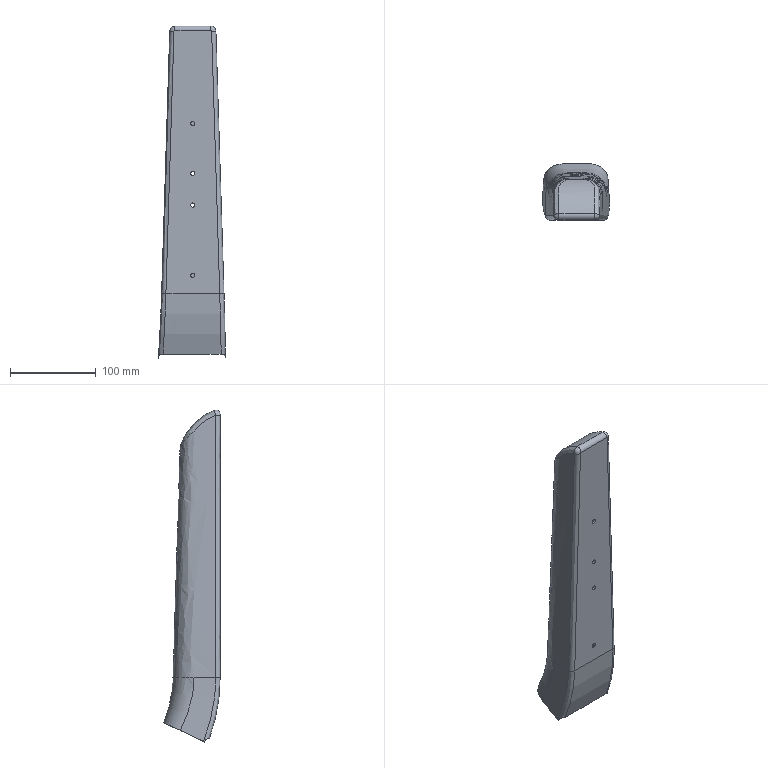Part | STEP file | Handlebar Cover L | 1 solid | 41 faces | box 78.327 x 65.639 x 387.41 mm | volume 737396 mm3 | spline 24 | cylinder 9 | plane 7 | torus 1 | commonest cylinder face diameters 5 x4 39 x2 7.5 x1 10 x1 137.836 x1